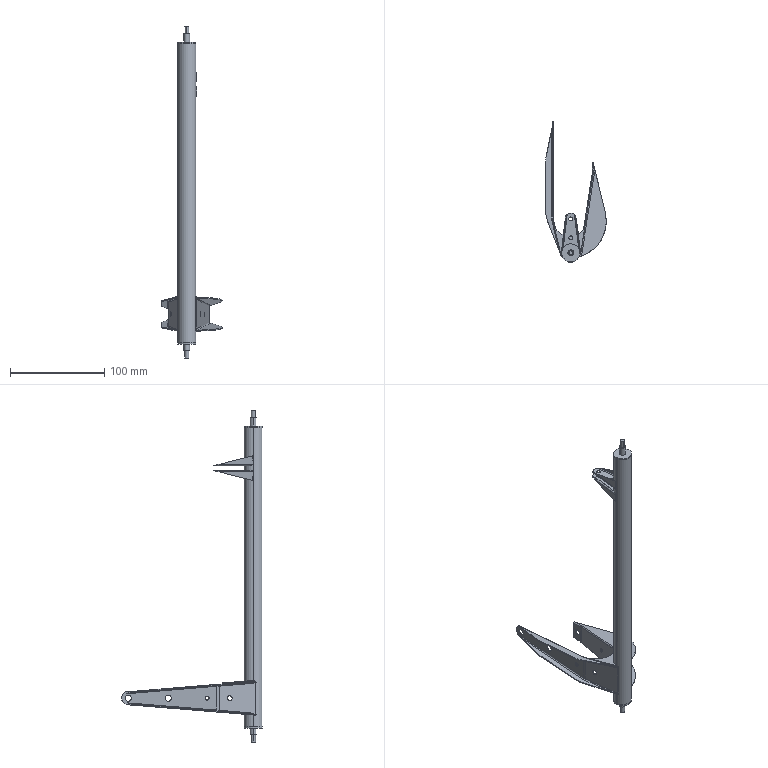Part | SolidWorks | features BaseBody 6 | 6 solids | 187 faces | box 64.263 x 148.912 x 351.5 mm | volume 29831 mm3 | cylinder 84 | plane 76 | spline 27 | commonest cylinder face diameters 2.032 x12 6.35 x10 19.05 x9 4.166 x8 2.54 x6 3.032 x4